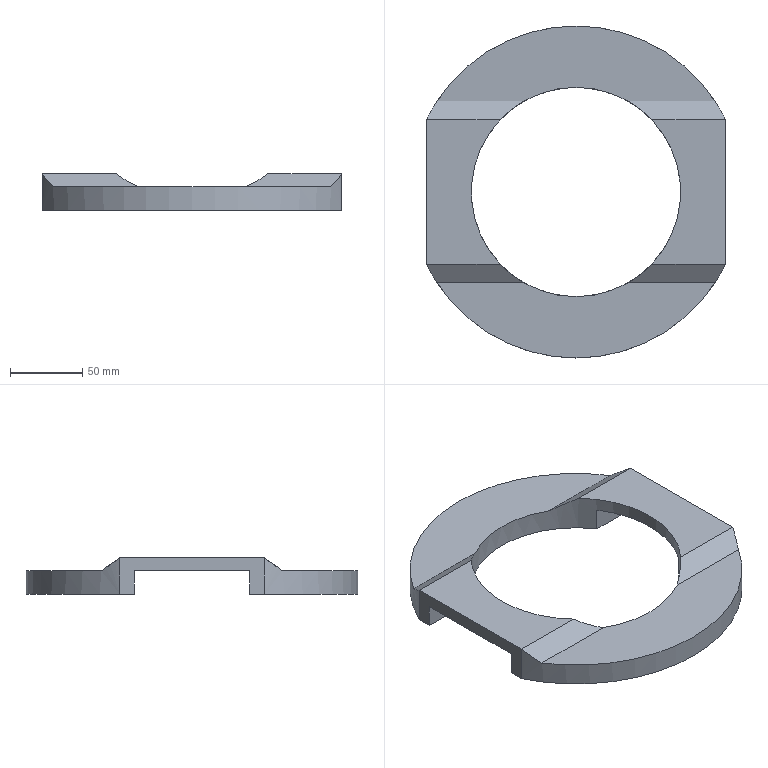Part | NX | features 掩护梁 2 | 1 solid | 21 faces | box 207.123 x 230 x 25 mm | volume 366015 mm3 | plane 18 | cylinder 3 | commonest cylinder face diameters 230 x2 145 x1
STEP:
#1=CARTESIAN_POINT('',(-1532.742,3715.447,718.229));
#2=VERTEX_POINT('',#1);
#3=CARTESIAN_POINT('',(-1532.742,3715.447,743.229));
#4=VERTEX_POINT('',#3);
#5=CARTESIAN_POINT('',(-1532.742,3715.447,743.229));
#6=DIRECTION('',(0.,0.,-1.));
#7=VECTOR('',#6,1000.);
#8=LINE('',#5,#7);
#9=EDGE_CURVE('',#2,#4,#8,.F.);
#10=ORIENTED_EDGE('',*,*,#9,.F.);
#11=CARTESIAN_POINT('',(-1325.619,3715.447,718.229));
#12=VERTEX_POINT('',#11);
#13=CARTESIAN_POINT('',(-1429.181,3765.447,718.229));
#14=DIRECTION('',(0.,0.,-1.));
#15=DIRECTION('',(-1.,0.,0.));
#16=AXIS2_PLACEMENT_3D('',#13,#14,#15);
#17=CIRCLE('',#16,115.);
#18=EDGE_CURVE('',#12,#2,#17,.T.);
#19=ORIENTED_EDGE('',*,*,#18,.F.);
#20=CARTESIAN_POINT('',(-1325.619,3715.447,743.229));
#21=VERTEX_POINT('',#20);
#22=CARTESIAN_POINT('',(-1325.619,3715.447,743.229));
#23=DIRECTION('',(0.,0.,-1.));
#24=VECTOR('',#23,1000.);
#25=LINE('',#22,#24);
#26=EDGE_CURVE('',#21,#12,#25,.T.);
#27=ORIENTED_EDGE('',*,*,#26,.F.);
#28=CARTESIAN_POINT('',(-1332.877,3702.594,734.229));
#29=VERTEX_POINT('',#28);
#30=CARTESIAN_POINT('',(-1429.181,3765.447,778.239));
#31=DIRECTION('',(0.,-0.5736,0.8192));
#32=DIRECTION('',(0.,-0.8192,-0.5736));
#33=AXIS2_PLACEMENT_3D('',#30,#31,#32);
#34=ELLIPSE('',#33,140.389,115.);
#35=EDGE_CURVE('',#21,#29,#34,.F.);
#36=ORIENTED_EDGE('',*,*,#35,.T.);
#37=CARTESIAN_POINT('',(-1525.485,3702.594,734.229));
#38=VERTEX_POINT('',#37);
#39=CARTESIAN_POINT('',(-1429.181,3765.447,734.229));
#40=DIRECTION('',(0.,0.,1.));
#41=DIRECTION('',(1.,0.,0.));
#42=AXIS2_PLACEMENT_3D('',#39,#40,#41);
#43=CIRCLE('',#42,115.);
#44=EDGE_CURVE('',#29,#38,#43,.F.);
#45=ORIENTED_EDGE('',*,*,#44,.T.);
#46=CARTESIAN_POINT('',(-1429.181,3765.447,778.239));
#47=DIRECTION('',(0.,-0.5736,0.8192));
#48=DIRECTION('',(0.,-0.8192,-0.5736));
#49=AXIS2_PLACEMENT_3D('',#46,#47,#48);
#50=ELLIPSE('',#49,140.389,115.);
#51=EDGE_CURVE('',#38,#4,#50,.F.);
#52=ORIENTED_EDGE('',*,*,#51,.T.);
#53=EDGE_LOOP('',(#10,#19,#27,#36,#45,#52));
#54=FACE_BOUND('',#53,.T.);
#55=CARTESIAN_POINT('',(-1429.181,3765.447,743.229));
#56=DIRECTION('',(0.,0.,-1.));
#57=DIRECTION('',(-1.,0.,0.));
#58=AXIS2_PLACEMENT_3D('',#55,#56,#57);
#59=CYLINDRICAL_SURFACE('',#58,115.);
#60=ADVANCED_FACE('',(#54),#59,.T.);
#61=CARTESIAN_POINT('',(-1532.742,3815.447,743.229));
#62=VERTEX_POINT('',#61);
#63=CARTESIAN_POINT('',(-1532.742,3815.447,718.229));
#64=VERTEX_POINT('',#63);
#65=CARTESIAN_POINT('',(-1532.742,3815.447,743.229));
#66=DIRECTION('',(0.,0.,-1.));
#67=VECTOR('',#66,1000.);
#68=LINE('',#65,#67);
#69=EDGE_CURVE('',#62,#64,#68,.T.);
#70=ORIENTED_EDGE('',*,*,#69,.F.);
#71=CARTESIAN_POINT('',(-1525.485,3828.301,734.229));
#72=VERTEX_POINT('',#71);
#73=CARTESIAN_POINT('',(-1429.181,3765.447,778.239));
#74=DIRECTION('',(0.,0.5736,0.8192));
#75=DIRECTION('',(0.,0.8192,-0.5736));
#76=AXIS2_PLACEMENT_3D('',#73,#74,#75);
#77=ELLIPSE('',#76,140.389,115.);
#78=EDGE_CURVE('',#62,#72,#77,.F.);
#79=ORIENTED_EDGE('',*,*,#78,.T.);
#80=CARTESIAN_POINT('',(-1332.877,3828.301,734.229));
#81=VERTEX_POINT('',#80);
#82=CARTESIAN_POINT('',(-1429.181,3765.447,734.229));
#83=DIRECTION('',(0.,0.,1.));
#84=DIRECTION('',(1.,0.,0.));
#85=AXIS2_PLACEMENT_3D('',#82,#83,#84);
#86=CIRCLE('',#85,115.);
#87=EDGE_CURVE('',#72,#81,#86,.F.);
#88=ORIENTED_EDGE('',*,*,#87,.T.);
#89=CARTESIAN_POINT('',(-1325.619,3815.447,743.229));
#90=VERTEX_POINT('',#89);
#91=CARTESIAN_POINT('',(-1429.181,3765.447,778.239));
#92=DIRECTION('',(0.,0.5736,0.8192));
#93=DIRECTION('',(0.,0.8192,-0.5736));
#94=AXIS2_PLACEMENT_3D('',#91,#92,#93);
#95=ELLIPSE('',#94,140.389,115.);
#96=EDGE_CURVE('',#81,#90,#95,.F.);
#97=ORIENTED_EDGE('',*,*,#96,.T.);
#98=CARTESIAN_POINT('',(-1325.619,3815.447,718.229));
#99=VERTEX_POINT('',#98);
#100=CARTESIAN_POINT('',(-1325.619,3815.447,743.229));
#101=DIRECTION('',(0.,0.,-1.));
#102=VECTOR('',#101,1000.);
#103=LINE('',#100,#102);
#104=EDGE_CURVE('',#99,#90,#103,.F.);
#105=ORIENTED_EDGE('',*,*,#104,.F.);
#106=CARTESIAN_POINT('',(-1429.181,3765.447,718.229));
#107=DIRECTION('',(0.,0.,-1.));
#108=DIRECTION('',(-1.,0.,0.));
#109=AXIS2_PLACEMENT_3D('',#106,#107,#108);
#110=CIRCLE('',#109,115.);
#111=EDGE_CURVE('',#64,#99,#110,.T.);
#112=ORIENTED_EDGE('',*,*,#111,.F.);
#113=EDGE_LOOP('',(#70,#79,#88,#97,#105,#112));
#114=FACE_BOUND('',#113,.T.);
#115=CARTESIAN_POINT('',(-1429.181,3765.447,743.229));
#116=DIRECTION('',(0.,0.,-1.));
#117=DIRECTION('',(-1.,0.,0.));
#118=AXIS2_PLACEMENT_3D('',#115,#116,#117);
#119=CYLINDRICAL_SURFACE('',#118,115.);
#120=ADVANCED_FACE('',(#114),#119,.T.);
#121=CARTESIAN_POINT('',(-1376.681,3715.447,743.229));
#122=VERTEX_POINT('',#121);
#123=CARTESIAN_POINT('',(-2112.181,3715.447,743.229));
#124=DIRECTION('',(1.,0.,0.));
#125=VECTOR('',#124,1000.);
#126=LINE('',#123,#125);
#127=EDGE_CURVE('',#122,#21,#126,.T.);
#128=ORIENTED_EDGE('',*,*,#127,.T.);
#129=CARTESIAN_POINT('',(-1325.619,3901.447,743.229));
#130=DIRECTION('',(0.,-1.,0.));
#131=VECTOR('',#130,1000.);
#132=LINE('',#129,#131);
#133=EDGE_CURVE('',#90,#21,#132,.T.);
#134=ORIENTED_EDGE('',*,*,#133,.F.);
#135=CARTESIAN_POINT('',(-1376.681,3815.447,743.229));
#136=VERTEX_POINT('',#135);
#137=CARTESIAN_POINT('',(-2112.181,3815.447,743.229));
#138=DIRECTION('',(1.,0.,0.));
#139=VECTOR('',#138,1000.);
#140=LINE('',#137,#139);
#141=EDGE_CURVE('',#136,#90,#140,.T.);
#142=ORIENTED_EDGE('',*,*,#141,.F.);
#143=CARTESIAN_POINT('',(-1429.181,3765.447,743.229));
#144=DIRECTION('',(0.,0.,-1.));
#145=DIRECTION('',(-1.,0.,0.));
#146=AXIS2_PLACEMENT_3D('',#143,#144,#145);
#147=CIRCLE('',#146,72.5);
#148=EDGE_CURVE('',#136,#122,#147,.T.);
#149=ORIENTED_EDGE('',*,*,#148,.T.);
#150=EDGE_LOOP('',(#128,#134,#142,#149));
#151=FACE_BOUND('',#150,.T.);
#152=CARTESIAN_POINT('',(-1429.181,3765.447,743.229));
#153=DIRECTION('',(0.,0.,-1.));
#154=DIRECTION('',(-1.,0.,0.));
#155=AXIS2_PLACEMENT_3D('',#152,#153,#154);
#156=PLANE('',#155);
#157=ADVANCED_FACE('',(#151),#156,.F.);
#158=CARTESIAN_POINT('',(-1481.681,3815.447,743.229));
#159=VERTEX_POINT('',#158);
#160=CARTESIAN_POINT('',(-2112.181,3815.447,743.229));
#161=DIRECTION('',(1.,0.,0.));
#162=VECTOR('',#161,1000.);
#163=LINE('',#160,#162);
#164=EDGE_CURVE('',#62,#159,#163,.T.);
#165=ORIENTED_EDGE('',*,*,#164,.F.);
#166=CARTESIAN_POINT('',(-1532.742,3901.447,743.229));
#167=DIRECTION('',(0.,-1.,0.));
#168=VECTOR('',#167,1000.);
#169=LINE('',#166,#168);
#170=EDGE_CURVE('',#62,#4,#169,.T.);
#171=ORIENTED_EDGE('',*,*,#170,.T.);
#172=CARTESIAN_POINT('',(-1481.681,3715.447,743.229));
#173=VERTEX_POINT('',#172);
#174=CARTESIAN_POINT('',(-2112.181,3715.447,743.229));
#175=DIRECTION('',(1.,0.,0.));
#176=VECTOR('',#175,1000.);
#177=LINE('',#174,#176);
#178=EDGE_CURVE('',#4,#173,#177,.T.);
#179=ORIENTED_EDGE('',*,*,#178,.T.);
#180=CARTESIAN_POINT('',(-1429.181,3765.447,743.229));
#181=DIRECTION('',(0.,0.,-1.));
#182=DIRECTION('',(-1.,0.,0.));
#183=AXIS2_PLACEMENT_3D('',#180,#181,#182);
#184=CIRCLE('',#183,72.5);
#185=EDGE_CURVE('',#173,#159,#184,.T.);
#186=ORIENTED_EDGE('',*,*,#185,.T.);
#187=EDGE_LOOP('',(#165,#171,#179,#186));
#188=FACE_BOUND('',#187,.T.);
#189=CARTESIAN_POINT('',(-1429.181,3765.447,743.229));
#190=DIRECTION('',(0.,0.,-1.));
#191=DIRECTION('',(-1.,0.,0.));
#192=AXIS2_PLACEMENT_3D('',#189,#190,#191);
#193=PLANE('',#192);
#194=ADVANCED_FACE('',(#188),#193,.F.);
#195=CARTESIAN_POINT('',(-1532.742,3725.447,718.229));
#196=VERTEX_POINT('',#195);
#197=CARTESIAN_POINT('',(-1532.742,3901.447,718.229));
#198=DIRECTION('',(0.,-1.,0.));
#199=VECTOR('',#198,1000.);
#200=LINE('',#197,#199);
#201=EDGE_CURVE('',#196,#2,#200,.T.);
#202=ORIENTED_EDGE('',*,*,#201,.F.);
#203=CARTESIAN_POINT('',(-1489.648,3725.447,718.229));
#204=VERTEX_POINT('',#203);
#205=CARTESIAN_POINT('',(-2112.181,3725.447,718.229));
#206=DIRECTION('',(1.,0.,0.));
#207=VECTOR('',#206,1000.);
#208=LINE('',#205,#207);
#209=EDGE_CURVE('',#196,#204,#208,.T.);
#210=ORIENTED_EDGE('',*,*,#209,.T.);
#211=CARTESIAN_POINT('',(-1368.714,3725.447,718.229));
#212=VERTEX_POINT('',#211);
#213=CARTESIAN_POINT('',(-1429.181,3765.447,718.229));
#214=DIRECTION('',(0.,0.,-1.));
#215=DIRECTION('',(-1.,0.,0.));
#216=AXIS2_PLACEMENT_3D('',#213,#214,#215);
#217=CIRCLE('',#216,72.5);
#218=EDGE_CURVE('',#212,#204,#217,.T.);
#219=ORIENTED_EDGE('',*,*,#218,.F.);
#220=CARTESIAN_POINT('',(-1325.619,3725.447,718.229));
#221=VERTEX_POINT('',#220);
#222=CARTESIAN_POINT('',(-2112.181,3725.447,718.229));
#223=DIRECTION('',(1.,0.,0.));
#224=VECTOR('',#223,1000.);
#225=LINE('',#222,#224);
#226=EDGE_CURVE('',#212,#221,#225,.T.);
#227=ORIENTED_EDGE('',*,*,#226,.T.);
#228=CARTESIAN_POINT('',(-1325.619,3901.447,718.229));
#229=DIRECTION('',(0.,-1.,0.));
#230=VECTOR('',#229,1000.);
#231=LINE('',#228,#230);
#232=EDGE_CURVE('',#221,#12,#231,.T.);
#233=ORIENTED_EDGE('',*,*,#232,.T.);
#234=ORIENTED_EDGE('',*,*,#18,.T.);
#235=EDGE_LOOP('',(#202,#210,#219,#227,#233,#234));
#236=FACE_BOUND('',#235,.T.);
#237=CARTESIAN_POINT('',(-1429.181,3765.447,718.229));
#238=DIRECTION('',(0.,0.,-1.));
#239=DIRECTION('',(-1.,0.,0.));
#240=AXIS2_PLACEMENT_3D('',#237,#238,#239);
#241=PLANE('',#240);
#242=ADVANCED_FACE('',(#236),#241,.T.);
#243=CARTESIAN_POINT('',(-1532.742,3805.447,718.229));
#244=VERTEX_POINT('',#243);
#245=CARTESIAN_POINT('',(-1532.742,3901.447,718.229));
#246=DIRECTION('',(0.,-1.,0.));
#247=VECTOR('',#246,1000.);
#248=LINE('',#245,#247);
#249=EDGE_CURVE('',#64,#244,#248,.T.);
#250=ORIENTED_EDGE('',*,*,#249,.F.);
#251=ORIENTED_EDGE('',*,*,#111,.T.);
#252=CARTESIAN_POINT('',(-1325.619,3805.447,718.229));
#253=VERTEX_POINT('',#252);
#254=CARTESIAN_POINT('',(-1325.619,3901.447,718.229));
#255=DIRECTION('',(0.,-1.,0.));
#256=VECTOR('',#255,1000.);
#257=LINE('',#254,#256);
#258=EDGE_CURVE('',#99,#253,#257,.T.);
#259=ORIENTED_EDGE('',*,*,#258,.T.);
#260=CARTESIAN_POINT('',(-1368.714,3805.447,718.229));
#261=VERTEX_POINT('',#260);
#262=CARTESIAN_POINT('',(-2112.181,3805.447,718.229));
#263=DIRECTION('',(1.,0.,0.));
#264=VECTOR('',#263,1000.);
#265=LINE('',#262,#264);
#266=EDGE_CURVE('',#261,#253,#265,.T.);
#267=ORIENTED_EDGE('',*,*,#266,.F.);
#268=CARTESIAN_POINT('',(-1489.648,3805.447,718.229));
#269=VERTEX_POINT('',#268);
#270=CARTESIAN_POINT('',(-1429.181,3765.447,718.229));
#271=DIRECTION('',(0.,0.,-1.));
#272=DIRECTION('',(-1.,0.,0.));
#273=AXIS2_PLACEMENT_3D('',#270,#271,#272);
#274=CIRCLE('',#273,72.5);
#275=EDGE_CURVE('',#269,#261,#274,.T.);
#276=ORIENTED_EDGE('',*,*,#275,.F.);
#277=CARTESIAN_POINT('',(-2112.181,3805.447,718.229));
#278=DIRECTION('',(1.,0.,0.));
#279=VECTOR('',#278,1000.);
#280=LINE('',#277,#279);
#281=EDGE_CURVE('',#244,#269,#280,.T.);
#282=ORIENTED_EDGE('',*,*,#281,.F.);
#283=EDGE_LOOP('',(#250,#251,#259,#267,#276,#282));
#284=FACE_BOUND('',#283,.T.);
#285=CARTESIAN_POINT('',(-1429.181,3765.447,718.229));
#286=DIRECTION('',(0.,0.,-1.));
#287=DIRECTION('',(-1.,0.,0.));
#288=AXIS2_PLACEMENT_3D('',#285,#286,#287);
#289=PLANE('',#288);
#290=ADVANCED_FACE('',(#284),#289,.T.);
#291=CARTESIAN_POINT('',(-1465.315,3702.594,734.229));
#292=VERTEX_POINT('',#291);
#293=CARTESIAN_POINT('',(-1429.181,3765.447,778.239));
#294=DIRECTION('',(0.,-0.5736,0.8192));
#295=DIRECTION('',(0.,-0.8192,-0.5736));
#296=AXIS2_PLACEMENT_3D('',#293,#294,#295);
#297=ELLIPSE('',#296,88.506,72.5);
#298=EDGE_CURVE('',#292,#173,#297,.F.);
#299=ORIENTED_EDGE('',*,*,#298,.F.);
#300=CARTESIAN_POINT('',(-1393.046,3702.594,734.229));
#301=VERTEX_POINT('',#300);
#302=CARTESIAN_POINT('',(-1429.181,3765.447,734.229));
#303=DIRECTION('',(0.,0.,1.));
#304=DIRECTION('',(1.,0.,0.));
#305=AXIS2_PLACEMENT_3D('',#302,#303,#304);
#306=CIRCLE('',#305,72.5);
#307=EDGE_CURVE('',#301,#292,#306,.F.);
#308=ORIENTED_EDGE('',*,*,#307,.F.);
#309=CARTESIAN_POINT('',(-1429.181,3765.447,778.239));
#310=DIRECTION('',(0.,-0.5736,0.8192));
#311=DIRECTION('',(0.,-0.8192,-0.5736));
#312=AXIS2_PLACEMENT_3D('',#309,#310,#311);
#313=ELLIPSE('',#312,88.506,72.5);
#314=EDGE_CURVE('',#122,#301,#313,.F.);
#315=ORIENTED_EDGE('',*,*,#314,.F.);
#316=ORIENTED_EDGE('',*,*,#148,.F.);
#317=CARTESIAN_POINT('',(-1393.046,3828.301,734.229));
#318=VERTEX_POINT('',#317);
#319=CARTESIAN_POINT('',(-1429.181,3765.447,778.239));
#320=DIRECTION('',(0.,0.5736,0.8192));
#321=DIRECTION('',(0.,0.8192,-0.5736));
#322=AXIS2_PLACEMENT_3D('',#319,#320,#321);
#323=ELLIPSE('',#322,88.506,72.5);
#324=EDGE_CURVE('',#318,#136,#323,.F.);
#325=ORIENTED_EDGE('',*,*,#324,.F.);
#326=CARTESIAN_POINT('',(-1465.315,3828.301,734.229));
#327=VERTEX_POINT('',#326);
#328=CARTESIAN_POINT('',(-1429.181,3765.447,734.229));
#329=DIRECTION('',(0.,0.,1.));
#330=DIRECTION('',(1.,0.,0.));
#331=AXIS2_PLACEMENT_3D('',#328,#329,#330);
#332=CIRCLE('',#331,72.5);
#333=EDGE_CURVE('',#327,#318,#332,.F.);
#334=ORIENTED_EDGE('',*,*,#333,.F.);
#335=CARTESIAN_POINT('',(-1429.181,3765.447,778.239));
#336=DIRECTION('',(0.,0.5736,0.8192));
#337=DIRECTION('',(0.,0.8192,-0.5736));
#338=AXIS2_PLACEMENT_3D('',#335,#336,#337);
#339=ELLIPSE('',#338,88.506,72.5);
#340=EDGE_CURVE('',#159,#327,#339,.F.);
#341=ORIENTED_EDGE('',*,*,#340,.F.);
#342=ORIENTED_EDGE('',*,*,#185,.F.);
#343=EDGE_LOOP('',(#299,#308,#315,#316,#325,#334,#341,#342));
#344=FACE_BOUND('',#343,.T.);
#345=CARTESIAN_POINT('',(-1489.648,3725.447,734.229));
#346=VERTEX_POINT('',#345);
#347=CARTESIAN_POINT('',(-1489.648,3725.447,743.229));
#348=DIRECTION('',(0.,0.,-1.));
#349=VECTOR('',#348,1000.);
#350=LINE('',#347,#349);
#351=EDGE_CURVE('',#346,#204,#350,.T.);
#352=ORIENTED_EDGE('',*,*,#351,.F.);
#353=CARTESIAN_POINT('',(-1489.648,3805.447,734.229));
#354=VERTEX_POINT('',#353);
#355=CARTESIAN_POINT('',(-1429.181,3765.447,734.229));
#356=DIRECTION('',(0.,0.,-1.));
#357=DIRECTION('',(-1.,0.,0.));
#358=AXIS2_PLACEMENT_3D('',#355,#356,#357);
#359=CIRCLE('',#358,72.5);
#360=EDGE_CURVE('',#354,#346,#359,.F.);
#361=ORIENTED_EDGE('',*,*,#360,.F.);
#362=CARTESIAN_POINT('',(-1489.648,3805.447,743.229));
#363=DIRECTION('',(0.,0.,-1.));
#364=VECTOR('',#363,1000.);
#365=LINE('',#362,#364);
#366=EDGE_CURVE('',#269,#354,#365,.F.);
#367=ORIENTED_EDGE('',*,*,#366,.F.);
#368=ORIENTED_EDGE('',*,*,#275,.T.);
#369=CARTESIAN_POINT('',(-1368.714,3805.447,734.229));
#370=VERTEX_POINT('',#369);
#371=CARTESIAN_POINT('',(-1368.714,3805.447,743.229));
#372=DIRECTION('',(0.,0.,-1.));
#373=VECTOR('',#372,1000.);
#374=LINE('',#371,#373);
#375=EDGE_CURVE('',#370,#261,#374,.T.);
#376=ORIENTED_EDGE('',*,*,#375,.F.);
#377=CARTESIAN_POINT('',(-1368.714,3725.447,734.229));
#378=VERTEX_POINT('',#377);
#379=CARTESIAN_POINT('',(-1429.181,3765.447,734.229));
#380=DIRECTION('',(0.,0.,-1.));
#381=DIRECTION('',(-1.,0.,0.));
#382=AXIS2_PLACEMENT_3D('',#379,#380,#381);
#383=CIRCLE('',#382,72.5);
#384=EDGE_CURVE('',#378,#370,#383,.F.);
#385=ORIENTED_EDGE('',*,*,#384,.F.);
#386=CARTESIAN_POINT('',(-1368.714,3725.447,743.229));
#387=DIRECTION('',(0.,0.,-1.));
#388=VECTOR('',#387,1000.);
#389=LINE('',#386,#388);
#390=EDGE_CURVE('',#212,#378,#389,.F.);
#391=ORIENTED_EDGE('',*,*,#390,.F.);
#392=ORIENTED_EDGE('',*,*,#218,.T.);
#393=EDGE_LOOP('',(#352,#361,#367,#368,#376,#385,#391,#392));
#394=FACE_BOUND('',#393,.T.);
#395=CARTESIAN_POINT('',(-1429.181,3765.447,743.229));
#396=DIRECTION('',(0.,0.,-1.));
#397=DIRECTION('',(-1.,0.,0.));
#398=AXIS2_PLACEMENT_3D('',#395,#396,#397);
#399=CYLINDRICAL_SURFACE('',#398,72.5);
#400=ADVANCED_FACE('',(#344,#394),#399,.F.);
#401=CARTESIAN_POINT('',(-2112.181,3828.301,734.229));
#402=DIRECTION('',(1.,0.,0.));
#403=VECTOR('',#402,1000.);
#404=LINE('',#401,#403);
#405=EDGE_CURVE('',#72,#327,#404,.T.);
#406=ORIENTED_EDGE('',*,*,#405,.T.);
#407=ORIENTED_EDGE('',*,*,#333,.T.);
#408=CARTESIAN_POINT('',(-2112.181,3828.301,734.229));
#409=DIRECTION('',(1.,0.,0.));
#410=VECTOR('',#409,1000.);
#411=LINE('',#408,#410);
#412=EDGE_CURVE('',#318,#81,#411,.T.);
#413=ORIENTED_EDGE('',*,*,#412,.T.);
#414=ORIENTED_EDGE('',*,*,#87,.F.);
#415=EDGE_LOOP('',(#406,#407,#413,#414));
#416=FACE_BOUND('',#415,.T.);
#417=CARTESIAN_POINT('',(-2112.181,3828.301,734.229));
#418=DIRECTION('',(0.,0.,1.));
#419=DIRECTION('',(1.,0.,0.));
#420=AXIS2_PLACEMENT_3D('',#417,#418,#419);
#421=PLANE('',#420);
#422=ADVANCED_FACE('',(#416),#421,.T.);
#423=ORIENTED_EDGE('',*,*,#412,.F.);
#424=ORIENTED_EDGE('',*,*,#324,.T.);
#425=ORIENTED_EDGE('',*,*,#141,.T.);
#426=ORIENTED_EDGE('',*,*,#96,.F.);
#427=EDGE_LOOP('',(#423,#424,#425,#426));
#428=FACE_BOUND('',#427,.T.);
#429=CARTESIAN_POINT('',(-2112.181,3815.447,743.229));
#430=DIRECTION('',(0.,0.5736,0.8192));
#431=DIRECTION('',(0.,-0.8192,0.5736));
#432=AXIS2_PLACEMENT_3D('',#429,#430,#431);
#433=PLANE('',#432);
#434=ADVANCED_FACE('',(#428),#433,.T.);
#435=ORIENTED_EDGE('',*,*,#164,.T.);
#436=ORIENTED_EDGE('',*,*,#340,.T.);
#437=ORIENTED_EDGE('',*,*,#405,.F.);
#438=ORIENTED_EDGE('',*,*,#78,.F.);
#439=EDGE_LOOP('',(#435,#436,#437,#438));
#440=FACE_BOUND('',#439,.T.);
#441=CARTESIAN_POINT('',(-2112.181,3815.447,743.229));
#442=DIRECTION('',(0.,0.5736,0.8192));
#443=DIRECTION('',(0.,-0.8192,0.5736));
#444=AXIS2_PLACEMENT_3D('',#441,#442,#443);
#445=PLANE('',#444);
#446=ADVANCED_FACE('',(#440),#445,.T.);
#447=CARTESIAN_POINT('',(-2112.181,3702.594,734.229));
#448=DIRECTION('',(1.,0.,0.));
#449=VECTOR('',#448,1000.);
#450=LINE('',#447,#449);
#451=EDGE_CURVE('',#38,#292,#450,.T.);
#452=ORIENTED_EDGE('',*,*,#451,.T.);
#453=ORIENTED_EDGE('',*,*,#298,.T.);
#454=ORIENTED_EDGE('',*,*,#178,.F.);
#455=ORIENTED_EDGE('',*,*,#51,.F.);
#456=EDGE_LOOP('',(#452,#453,#454,#455));
#457=FACE_BOUND('',#456,.T.);
#458=CARTESIAN_POINT('',(-2112.181,3715.447,743.229));
#459=DIRECTION('',(0.,-0.5736,0.8192));
#460=DIRECTION('',(0.,-0.8192,-0.5736));
#461=AXIS2_PLACEMENT_3D('',#458,#459,#460);
#462=PLANE('',#461);
#463=ADVANCED_FACE('',(#457),#462,.T.);
#464=ORIENTED_EDGE('',*,*,#127,.F.);
#465=ORIENTED_EDGE('',*,*,#314,.T.);
#466=CARTESIAN_POINT('',(-2112.181,3702.594,734.229));
#467=DIRECTION('',(1.,0.,0.));
#468=VECTOR('',#467,1000.);
#469=LINE('',#466,#468);
#470=EDGE_CURVE('',#301,#29,#469,.T.);
#471=ORIENTED_EDGE('',*,*,#470,.T.);
#472=ORIENTED_EDGE('',*,*,#35,.F.);
#473=EDGE_LOOP('',(#464,#465,#471,#472));
#474=FACE_BOUND('',#473,.T.);
#475=CARTESIAN_POINT('',(-2112.181,3715.447,743.229));
#476=DIRECTION('',(0.,-0.5736,0.8192));
#477=DIRECTION('',(0.,-0.8192,-0.5736));
#478=AXIS2_PLACEMENT_3D('',#475,#476,#477);
#479=PLANE('',#478);
#480=ADVANCED_FACE('',(#474),#479,.T.);
#481=ORIENTED_EDGE('',*,*,#470,.F.);
#482=ORIENTED_EDGE('',*,*,#307,.T.);
#483=ORIENTED_EDGE('',*,*,#451,.F.);
#484=ORIENTED_EDGE('',*,*,#44,.F.);
#485=EDGE_LOOP('',(#481,#482,#483,#484));
#486=FACE_BOUND('',#485,.T.);
#487=CARTESIAN_POINT('',(-2112.181,3702.594,734.229));
#488=DIRECTION('',(0.,0.,1.));
#489=DIRECTION('',(1.,0.,0.));
#490=AXIS2_PLACEMENT_3D('',#487,#488,#489);
#491=PLANE('',#490);
#492=ADVANCED_FACE('',(#486),#491,.T.);
#493=CARTESIAN_POINT('',(-1325.619,3805.447,734.229));
#494=VERTEX_POINT('',#493);
#495=CARTESIAN_POINT('',(-1325.619,3805.447,734.229));
#496=DIRECTION('',(0.,0.,-1.));
#497=VECTOR('',#496,1000.);
#498=LINE('',#495,#497);
#499=EDGE_CURVE('',#494,#253,#498,.T.);
#500=ORIENTED_EDGE('',*,*,#499,.F.);
#501=CARTESIAN_POINT('',(-2112.181,3805.447,734.229));
#502=DIRECTION('',(1.,0.,0.));
#503=VECTOR('',#502,1000.);
#504=LINE('',#501,#503);
#505=EDGE_CURVE('',#370,#494,#504,.T.);
#506=ORIENTED_EDGE('',*,*,#505,.F.);
#507=ORIENTED_EDGE('',*,*,#375,.T.);
#508=ORIENTED_EDGE('',*,*,#266,.T.);
#509=EDGE_LOOP('',(#500,#506,#507,#508));
#510=FACE_BOUND('',#509,.T.);
#511=CARTESIAN_POINT('',(-2112.181,3805.447,734.229));
#512=DIRECTION('',(0.,-1.,0.));
#513=DIRECTION('',(0.,0.,-1.));
#514=AXIS2_PLACEMENT_3D('',#511,#512,#513);
#515=PLANE('',#514);
#516=ADVANCED_FACE('',(#510),#515,.T.);
#517=CARTESIAN_POINT('',(-1325.619,3725.447,734.229));
#518=VERTEX_POINT('',#517);
#519=CARTESIAN_POINT('',(-1325.619,3805.447,734.229));
#520=DIRECTION('',(0.,1.,0.));
#521=VECTOR('',#520,1000.);
#522=LINE('',#519,#521);
#523=EDGE_CURVE('',#518,#494,#522,.T.);
#524=ORIENTED_EDGE('',*,*,#523,.F.);
#525=CARTESIAN_POINT('',(-2112.181,3725.447,734.229));
#526=DIRECTION('',(1.,0.,0.));
#527=VECTOR('',#526,1000.);
#528=LINE('',#525,#527);
#529=EDGE_CURVE('',#378,#518,#528,.T.);
#530=ORIENTED_EDGE('',*,*,#529,.F.);
#531=ORIENTED_EDGE('',*,*,#384,.T.);
#532=ORIENTED_EDGE('',*,*,#505,.T.);
#533=EDGE_LOOP('',(#524,#530,#531,#532));
#534=FACE_BOUND('',#533,.T.);
#535=CARTESIAN_POINT('',(-2112.181,3805.447,734.229));
#536=DIRECTION('',(0.,0.,-1.));
#537=DIRECTION('',(-1.,0.,0.));
#538=AXIS2_PLACEMENT_3D('',#535,#536,#537);
#539=PLANE('',#538);
#540=ADVANCED_FACE('',(#534),#539,.T.);
#541=CARTESIAN_POINT('',(-1325.619,3725.447,734.229));
#542=DIRECTION('',(0.,0.,1.));
#543=VECTOR('',#542,1000.);
#544=LINE('',#541,#543);
#545=EDGE_CURVE('',#221,#518,#544,.T.);
#546=ORIENTED_EDGE('',*,*,#545,.F.);
#547=ORIENTED_EDGE('',*,*,#226,.F.);
#548=ORIENTED_EDGE('',*,*,#390,.T.);
#549=ORIENTED_EDGE('',*,*,#529,.T.);
#550=EDGE_LOOP('',(#546,#547,#548,#549));
#551=FACE_BOUND('',#550,.T.);
#552=CARTESIAN_POINT('',(-2112.181,3725.447,734.229));
#553=DIRECTION('',(0.,1.,0.));
#554=DIRECTION('',(0.,0.,1.));
#555=AXIS2_PLACEMENT_3D('',#552,#553,#554);
#556=PLANE('',#555);
#557=ADVANCED_FACE('',(#551),#556,.T.);
#558=CARTESIAN_POINT('',(-1532.742,3725.447,734.229));
#559=VERTEX_POINT('',#558);
#560=CARTESIAN_POINT('',(-1532.742,3725.447,734.229));
#561=DIRECTION('',(0.,0.,-1.));
#562=VECTOR('',#561,1000.);
#563=LINE('',#560,#562);
#564=EDGE_CURVE('',#559,#196,#563,.T.);
#565=ORIENTED_EDGE('',*,*,#564,.F.);
#566=CARTESIAN_POINT('',(-2112.181,3725.447,734.229));
#567=DIRECTION('',(1.,0.,0.));
#568=VECTOR('',#567,1000.);
#569=LINE('',#566,#568);
#570=EDGE_CURVE('',#559,#346,#569,.T.);
#571=ORIENTED_EDGE('',*,*,#570,.T.);
#572=ORIENTED_EDGE('',*,*,#351,.T.);
#573=ORIENTED_EDGE('',*,*,#209,.F.);
#574=EDGE_LOOP('',(#565,#571,#572,#573));
#575=FACE_BOUND('',#574,.T.);
#576=CARTESIAN_POINT('',(-2112.181,3725.447,734.229));
#577=DIRECTION('',(0.,1.,0.));
#578=DIRECTION('',(0.,0.,1.));
#579=AXIS2_PLACEMENT_3D('',#576,#577,#578);
#580=PLANE('',#579);
#581=ADVANCED_FACE('',(#575),#580,.T.);
#582=CARTESIAN_POINT('',(-1532.742,3805.447,734.229));
#583=VERTEX_POINT('',#582);
#584=CARTESIAN_POINT('',(-1532.742,3805.447,734.229));
#585=DIRECTION('',(0.,-1.,0.));
#586=VECTOR('',#585,1000.);
#587=LINE('',#584,#586);
#588=EDGE_CURVE('',#583,#559,#587,.T.);
#589=ORIENTED_EDGE('',*,*,#588,.F.);
#590=CARTESIAN_POINT('',(-2112.181,3805.447,734.229));
#591=DIRECTION('',(1.,0.,0.));
#592=VECTOR('',#591,1000.);
#593=LINE('',#590,#592);
#594=EDGE_CURVE('',#583,#354,#593,.T.);
#595=ORIENTED_EDGE('',*,*,#594,.T.);
#596=ORIENTED_EDGE('',*,*,#360,.T.);
#597=ORIENTED_EDGE('',*,*,#570,.F.);
#598=EDGE_LOOP('',(#589,#595,#596,#597));
#599=FACE_BOUND('',#598,.T.);
#600=CARTESIAN_POINT('',(-2112.181,3805.447,734.229));
#601=DIRECTION('',(0.,0.,-1.));
#602=DIRECTION('',(-1.,0.,0.));
#603=AXIS2_PLACEMENT_3D('',#600,#601,#602);
#604=PLANE('',#603);
#605=ADVANCED_FACE('',(#599),#604,.T.);
#606=CARTESIAN_POINT('',(-1532.742,3805.447,734.229));
#607=DIRECTION('',(0.,0.,1.));
#608=VECTOR('',#607,1000.);
#609=LINE('',#606,#608);
#610=EDGE_CURVE('',#244,#583,#609,.T.);
#611=ORIENTED_EDGE('',*,*,#610,.F.);
#612=ORIENTED_EDGE('',*,*,#281,.T.);
#613=ORIENTED_EDGE('',*,*,#366,.T.);
#614=ORIENTED_EDGE('',*,*,#594,.F.);
#615=EDGE_LOOP('',(#611,#612,#613,#614));
#616=FACE_BOUND('',#615,.T.);
#617=CARTESIAN_POINT('',(-2112.181,3805.447,734.229));
#618=DIRECTION('',(0.,-1.,0.));
#619=DIRECTION('',(0.,0.,-1.));
#620=AXIS2_PLACEMENT_3D('',#617,#618,#619);
#621=PLANE('',#620);
#622=ADVANCED_FACE('',(#616),#621,.T.);
#623=ORIENTED_EDGE('',*,*,#9,.T.);
#624=ORIENTED_EDGE('',*,*,#170,.F.);
#625=ORIENTED_EDGE('',*,*,#69,.T.);
#626=ORIENTED_EDGE('',*,*,#249,.T.);
#627=ORIENTED_EDGE('',*,*,#610,.T.);
#628=ORIENTED_EDGE('',*,*,#588,.T.);
#629=ORIENTED_EDGE('',*,*,#564,.T.);
#630=ORIENTED_EDGE('',*,*,#201,.T.);
#631=EDGE_LOOP('',(#623,#624,#625,#626,#627,#628,#629,#630));
#632=FACE_BOUND('',#631,.T.);
#633=CARTESIAN_POINT('',(-1532.742,3901.447,743.229));
#634=DIRECTION('',(1.,0.,0.));
#635=DIRECTION('',(0.,0.,-1.));
#636=AXIS2_PLACEMENT_3D('',#633,#634,#635);
#637=PLANE('',#636);
#638=ADVANCED_FACE('',(#632),#637,.F.);
#639=ORIENTED_EDGE('',*,*,#104,.T.);
#640=ORIENTED_EDGE('',*,*,#133,.T.);
#641=ORIENTED_EDGE('',*,*,#26,.T.);
#642=ORIENTED_EDGE('',*,*,#232,.F.);
#643=ORIENTED_EDGE('',*,*,#545,.T.);
#644=ORIENTED_EDGE('',*,*,#523,.T.);
#645=ORIENTED_EDGE('',*,*,#499,.T.);
#646=ORIENTED_EDGE('',*,*,#258,.F.);
#647=EDGE_LOOP('',(#639,#640,#641,#642,#643,#644,#645,#646));
#648=FACE_BOUND('',#647,.T.);
#649=CARTESIAN_POINT('',(-1325.619,3901.447,743.229));
#650=DIRECTION('',(-1.,0.,0.));
#651=DIRECTION('',(0.,0.,1.));
#652=AXIS2_PLACEMENT_3D('',#649,#650,#651);
#653=PLANE('',#652);
#654=ADVANCED_FACE('',(#648),#653,.F.);
#655=CLOSED_SHELL('',(#60,#120,#157,#194,#242,#290,#400,#422,#434,#446,#463,#480,#492,#516,#540,#557,#581,#605,#622,#638,#654));
#656=MANIFOLD_SOLID_BREP('',#655);
#657=(LENGTH_UNIT()NAMED_UNIT(*)SI_UNIT(.MILLI.,.METRE.));
#658=UNCERTAINTY_MEASURE_WITH_UNIT(LENGTH_MEASURE(0.00001),#657,'','');
#659=(NAMED_UNIT(*)PLANE_ANGLE_UNIT()SI_UNIT($,.RADIAN.));
#660=(NAMED_UNIT(*)SI_UNIT($,.STERADIAN.)SOLID_ANGLE_UNIT());
#661=(GEOMETRIC_REPRESENTATION_CONTEXT(3)GLOBAL_UNCERTAINTY_ASSIGNED_CONTEXT((#658))GLOBAL_UNIT_ASSIGNED_CONTEXT((#657,#659,#660))REPRESENTATION_CONTEXT('',''));
#662=ADVANCED_BREP_SHAPE_REPRESENTATION('',(#656),#661);